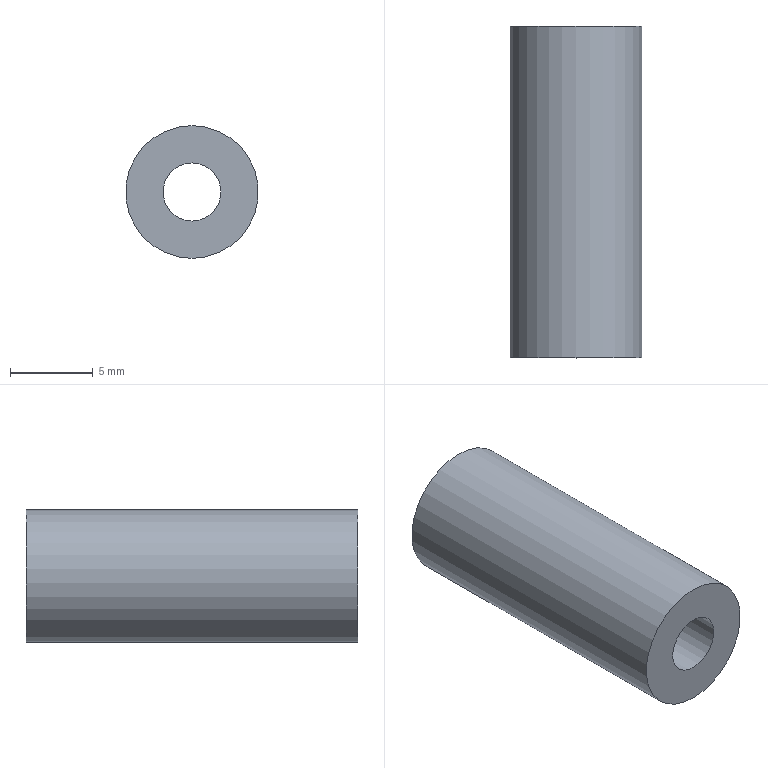Part | STEP file | lll_id4710_x_t | 1 solid | 4 faces | box 8 x 20 x 8 mm | volume 812.887 mm3 | cylinder 2 | plane 2 | commonest cylinder face diameters 3.5 x1 8 x1
STEP:
#1=CARTESIAN_POINT('',(785.37,-362.421,10.5));
#2=VERTEX_POINT('',#1);
#3=CARTESIAN_POINT('',(785.37,-362.421,14.5));
#4=DIRECTION('',(0.,1.,0.));
#5=DIRECTION('',(0.,0.,-1.));
#6=AXIS2_PLACEMENT_3D('',#3,#4,#5);
#7=CIRCLE('',#6,4.);
#8=EDGE_CURVE('',#2,#2,#7,.T.);
#9=ORIENTED_EDGE('',*,*,#8,.F.);
#10=EDGE_LOOP('',(#9));
#11=FACE_BOUND('',#10,.T.);
#12=CARTESIAN_POINT('',(785.37,-382.421,18.5));
#13=VERTEX_POINT('',#12);
#14=CARTESIAN_POINT('',(785.37,-382.421,14.5));
#15=DIRECTION('',(0.,1.,0.));
#16=DIRECTION('',(0.,0.,1.));
#17=AXIS2_PLACEMENT_3D('',#14,#15,#16);
#18=CIRCLE('',#17,4.);
#19=EDGE_CURVE('',#13,#13,#18,.T.);
#20=ORIENTED_EDGE('',*,*,#19,.T.);
#21=EDGE_LOOP('',(#20));
#22=FACE_BOUND('',#21,.T.);
#23=CARTESIAN_POINT('',(785.37,-345.421,14.5));
#24=DIRECTION('',(0.,-1.,0.));
#25=DIRECTION('',(0.,0.,-1.));
#26=AXIS2_PLACEMENT_3D('',#23,#24,#25);
#27=CYLINDRICAL_SURFACE('',#26,4.);
#28=ADVANCED_FACE('',(#11,#22),#27,.T.);
#29=CARTESIAN_POINT('',(785.37,-362.421,12.75));
#30=VERTEX_POINT('',#29);
#31=CARTESIAN_POINT('',(785.37,-362.421,14.5));
#32=DIRECTION('',(0.,-1.,0.));
#33=DIRECTION('',(0.,0.,-1.));
#34=AXIS2_PLACEMENT_3D('',#31,#32,#33);
#35=CIRCLE('',#34,1.75);
#36=EDGE_CURVE('',#30,#30,#35,.T.);
#37=ORIENTED_EDGE('',*,*,#36,.T.);
#38=EDGE_LOOP('',(#37));
#39=FACE_BOUND('',#38,.T.);
#40=ORIENTED_EDGE('',*,*,#8,.T.);
#41=EDGE_LOOP('',(#40));
#42=FACE_BOUND('',#41,.T.);
#43=CARTESIAN_POINT('',(785.37,-362.421,12.));
#44=DIRECTION('',(0.,-1.,0.));
#45=DIRECTION('',(0.,0.,-1.));
#46=AXIS2_PLACEMENT_3D('',#43,#44,#45);
#47=PLANE('',#46);
#48=ADVANCED_FACE('',(#39,#42),#47,.F.);
#49=CARTESIAN_POINT('',(785.37,-382.421,16.25));
#50=VERTEX_POINT('',#49);
#51=CARTESIAN_POINT('',(785.37,-382.421,14.5));
#52=DIRECTION('',(0.,1.,0.));
#53=DIRECTION('',(0.,0.,1.));
#54=AXIS2_PLACEMENT_3D('',#51,#52,#53);
#55=CIRCLE('',#54,1.75);
#56=EDGE_CURVE('',#50,#50,#55,.T.);
#57=ORIENTED_EDGE('',*,*,#56,.T.);
#58=EDGE_LOOP('',(#57));
#59=FACE_BOUND('',#58,.T.);
#60=ORIENTED_EDGE('',*,*,#19,.F.);
#61=EDGE_LOOP('',(#60));
#62=FACE_BOUND('',#61,.T.);
#63=CARTESIAN_POINT('',(785.37,-382.421,14.5));
#64=DIRECTION('',(0.,1.,0.));
#65=DIRECTION('',(0.,0.,1.));
#66=AXIS2_PLACEMENT_3D('',#63,#64,#65);
#67=PLANE('',#66);
#68=ADVANCED_FACE('',(#59,#62),#67,.F.);
#69=ORIENTED_EDGE('',*,*,#36,.F.);
#70=EDGE_LOOP('',(#69));
#71=FACE_BOUND('',#70,.T.);
#72=ORIENTED_EDGE('',*,*,#56,.F.);
#73=EDGE_LOOP('',(#72));
#74=FACE_BOUND('',#73,.T.);
#75=CARTESIAN_POINT('',(785.37,-362.421,14.5));
#76=DIRECTION('',(0.,-1.,0.));
#77=DIRECTION('',(0.,0.,-1.));
#78=AXIS2_PLACEMENT_3D('',#75,#76,#77);
#79=CYLINDRICAL_SURFACE('',#78,1.75);
#80=ADVANCED_FACE('',(#71,#74),#79,.F.);
#81=CLOSED_SHELL('',(#28,#48,#68,#80));
#82=MANIFOLD_SOLID_BREP('',#81);
#83=(LENGTH_UNIT()NAMED_UNIT(*)SI_UNIT(.MILLI.,.METRE.));
#84=UNCERTAINTY_MEASURE_WITH_UNIT(LENGTH_MEASURE(0.00002),#83,'','');
#85=(NAMED_UNIT(*)PLANE_ANGLE_UNIT()SI_UNIT($,.RADIAN.));
#86=PLANE_ANGLE_MEASURE_WITH_UNIT(PLANE_ANGLE_MEASURE(0.01745),#85);
#87=DIMENSIONAL_EXPONENTS(0.,0.,0.,0.,0.,0.,0.);
#88=(CONVERSION_BASED_UNIT('DEGREE',#86)NAMED_UNIT(#87)PLANE_ANGLE_UNIT());
#89=(NAMED_UNIT(*)SI_UNIT($,.STERADIAN.)SOLID_ANGLE_UNIT());
#90=(GEOMETRIC_REPRESENTATION_CONTEXT(3)GLOBAL_UNCERTAINTY_ASSIGNED_CONTEXT((#84))GLOBAL_UNIT_ASSIGNED_CONTEXT((#83,#88,#89))REPRESENTATION_CONTEXT('',''));
#91=ADVANCED_BREP_SHAPE_REPRESENTATION('',(#82),#90);